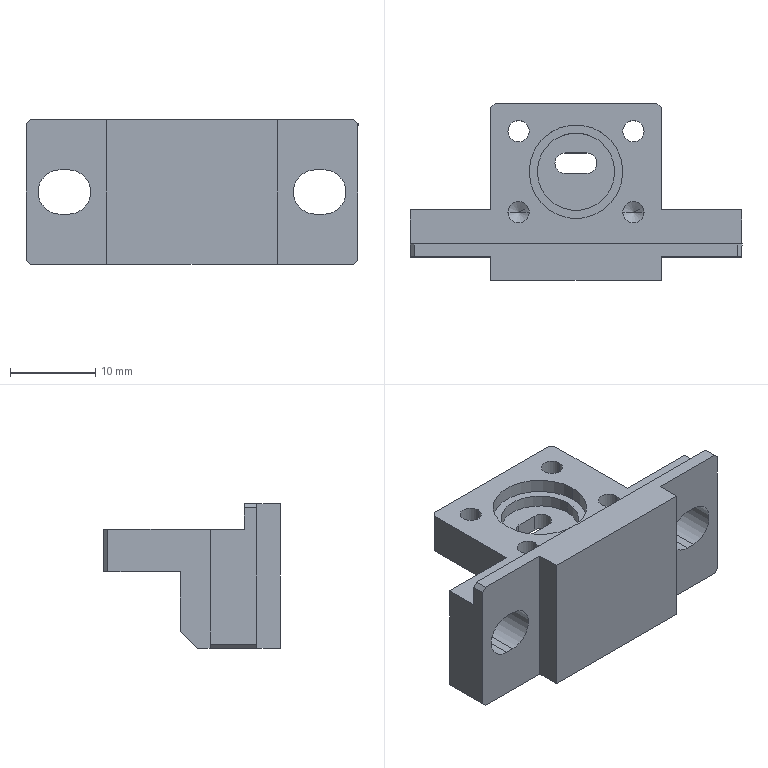Part | SolidWorks | features ICE 25, MoveFace 17, Chamfer 4, 3DProfileFeature 2, Fillet 2, HoleWzd 2, Extrusion 1, MirrorPattern 1 | 1 solid | 60 faces | box 39 x 20.75 x 17 mm | volume 5257 mm3 | plane 33 | cylinder 21 | cone 6 | commonest cylinder face diameters 2.5 x8 5.2 x4 2.4 x3 2 x2 9.1 x2 11 x2